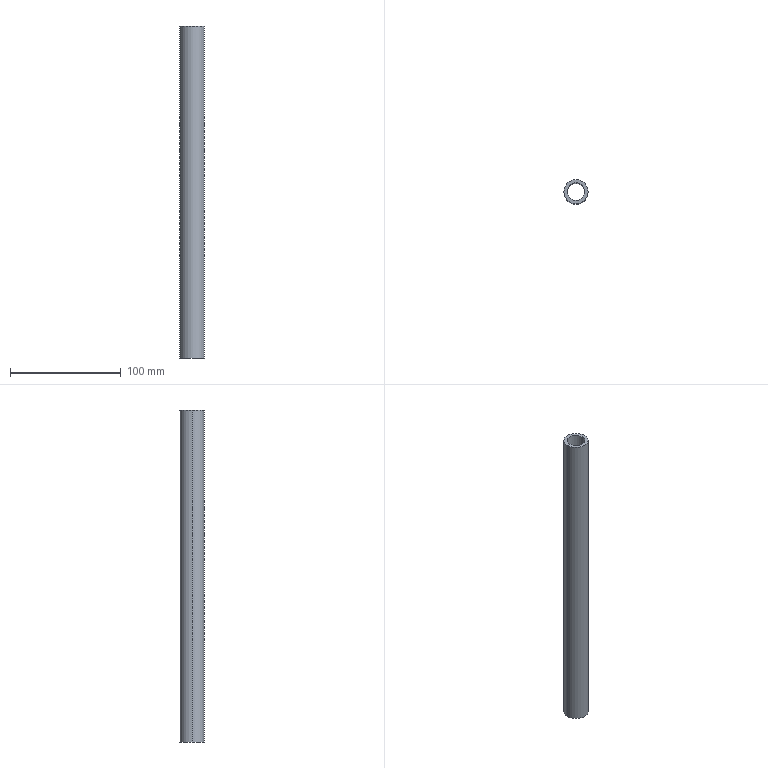Part | STEP file | 51E-01164JG10 | 1 solid | 6 faces | box 22 x 22 x 300 mm | volume 53721 mm3 | cylinder 4 | plane 2 | commonest cylinder face diameters 16 x2 22 x2
STEP:
#1=CARTESIAN_POINT('',(-8.,0.,150.));
#2=VERTEX_POINT('',#1);
#3=CARTESIAN_POINT('',(8.,0.,150.));
#4=VERTEX_POINT('',#3);
#5=CARTESIAN_POINT('',(0.,0.,150.));
#6=DIRECTION('',(0.,0.,-1.));
#7=AXIS2_PLACEMENT_3D('',#5,#6,$);
#8=CIRCLE('',#7,8.);
#9=EDGE_CURVE('',#2,#4,#8,.F.);
#10=ORIENTED_EDGE('',*,*,#9,.T.);
#11=CARTESIAN_POINT('',(8.,0.,-150.));
#12=VERTEX_POINT('',#11);
#13=CARTESIAN_POINT('',(8.,0.,150.));
#14=DIRECTION('',(0.,0.,-1.));
#15=VECTOR('',#14,1.);
#16=LINE('',#13,#15);
#17=EDGE_CURVE('',#4,#12,#16,.T.);
#18=ORIENTED_EDGE('',*,*,#17,.T.);
#19=CARTESIAN_POINT('',(-8.,0.,-150.));
#20=VERTEX_POINT('',#19);
#21=CARTESIAN_POINT('',(0.,0.,-150.));
#22=DIRECTION('',(0.,0.,-1.));
#23=AXIS2_PLACEMENT_3D('',#21,#22,$);
#24=CIRCLE('',#23,8.);
#25=EDGE_CURVE('',#20,#12,#24,.F.);
#26=ORIENTED_EDGE('',*,*,#25,.F.);
#27=CARTESIAN_POINT('',(-8.,0.,150.));
#28=DIRECTION('',(0.,0.,-1.));
#29=VECTOR('',#28,1.);
#30=LINE('',#27,#29);
#31=EDGE_CURVE('',#2,#20,#30,.T.);
#32=ORIENTED_EDGE('',*,*,#31,.F.);
#33=EDGE_LOOP('',(#10,#18,#26,#32));
#34=FACE_OUTER_BOUND('',#33,.T.);
#35=CARTESIAN_POINT('',(0.,0.,150.));
#36=DIRECTION('',(0.,0.,-1.));
#37=DIRECTION('',(1.,0.,0.));
#38=AXIS2_PLACEMENT_3D('',#35,#36,#37);
#39=CYLINDRICAL_SURFACE('',#38,8.);
#40=ADVANCED_FACE('',(#34),#39,.F.);
#41=CARTESIAN_POINT('',(-11.,0.,150.));
#42=VERTEX_POINT('',#41);
#43=CARTESIAN_POINT('',(11.,0.,150.));
#44=VERTEX_POINT('',#43);
#45=CARTESIAN_POINT('',(0.,0.,150.));
#46=DIRECTION('',(0.,0.,1.));
#47=AXIS2_PLACEMENT_3D('',#45,#46,$);
#48=CIRCLE('',#47,11.);
#49=EDGE_CURVE('',#42,#44,#48,.T.);
#50=ORIENTED_EDGE('',*,*,#49,.T.);
#51=CARTESIAN_POINT('',(0.,0.,150.));
#52=DIRECTION('',(0.,0.,1.));
#53=AXIS2_PLACEMENT_3D('',#51,#52,$);
#54=CIRCLE('',#53,11.);
#55=EDGE_CURVE('',#44,#42,#54,.T.);
#56=ORIENTED_EDGE('',*,*,#55,.T.);
#57=EDGE_LOOP('',(#50,#56));
#58=FACE_OUTER_BOUND('',#57,.T.);
#59=ORIENTED_EDGE('',*,*,#9,.F.);
#60=CARTESIAN_POINT('',(0.,0.,150.));
#61=DIRECTION('',(0.,0.,1.));
#62=AXIS2_PLACEMENT_3D('',#60,#61,$);
#63=CIRCLE('',#62,8.);
#64=EDGE_CURVE('',#4,#2,#63,.T.);
#65=ORIENTED_EDGE('',*,*,#64,.F.);
#66=EDGE_LOOP('',(#59,#65));
#67=FACE_BOUND('',#66,.T.);
#68=CARTESIAN_POINT('',(0.,0.,150.));
#69=DIRECTION('',(0.,0.,1.));
#70=DIRECTION('',(1.,0.,0.));
#71=AXIS2_PLACEMENT_3D('',#68,#69,#70);
#72=PLANE('',#71);
#73=ADVANCED_FACE('',(#58,#67),#72,.T.);
#74=ORIENTED_EDGE('',*,*,#17,.F.);
#75=ORIENTED_EDGE('',*,*,#64,.T.);
#76=ORIENTED_EDGE('',*,*,#31,.T.);
#77=CARTESIAN_POINT('',(0.,0.,-150.));
#78=DIRECTION('',(0.,0.,-1.));
#79=AXIS2_PLACEMENT_3D('',#77,#78,$);
#80=CIRCLE('',#79,8.);
#81=EDGE_CURVE('',#12,#20,#80,.F.);
#82=ORIENTED_EDGE('',*,*,#81,.F.);
#83=EDGE_LOOP('',(#74,#75,#76,#82));
#84=FACE_OUTER_BOUND('',#83,.T.);
#85=CARTESIAN_POINT('',(0.,0.,150.));
#86=DIRECTION('',(0.,0.,-1.));
#87=DIRECTION('',(-1.,0.,0.));
#88=AXIS2_PLACEMENT_3D('',#85,#86,#87);
#89=CYLINDRICAL_SURFACE('',#88,8.);
#90=ADVANCED_FACE('',(#84),#89,.F.);
#91=CARTESIAN_POINT('',(-11.,0.,-150.));
#92=VERTEX_POINT('',#91);
#93=CARTESIAN_POINT('',(11.,0.,-150.));
#94=VERTEX_POINT('',#93);
#95=CARTESIAN_POINT('',(0.,0.,-150.));
#96=DIRECTION('',(0.,0.,1.));
#97=AXIS2_PLACEMENT_3D('',#95,#96,$);
#98=CIRCLE('',#97,11.);
#99=EDGE_CURVE('',#92,#94,#98,.T.);
#100=ORIENTED_EDGE('',*,*,#99,.F.);
#101=CARTESIAN_POINT('',(0.,0.,-150.));
#102=DIRECTION('',(0.,0.,1.));
#103=AXIS2_PLACEMENT_3D('',#101,#102,$);
#104=CIRCLE('',#103,11.);
#105=EDGE_CURVE('',#94,#92,#104,.T.);
#106=ORIENTED_EDGE('',*,*,#105,.F.);
#107=EDGE_LOOP('',(#100,#106));
#108=FACE_OUTER_BOUND('',#107,.T.);
#109=ORIENTED_EDGE('',*,*,#25,.T.);
#110=ORIENTED_EDGE('',*,*,#81,.T.);
#111=EDGE_LOOP('',(#109,#110));
#112=FACE_BOUND('',#111,.T.);
#113=CARTESIAN_POINT('',(0.,0.,-150.));
#114=DIRECTION('',(0.,0.,1.));
#115=DIRECTION('',(1.,0.,0.));
#116=AXIS2_PLACEMENT_3D('',#113,#114,#115);
#117=PLANE('',#116);
#118=ADVANCED_FACE('',(#108,#112),#117,.F.);
#119=CARTESIAN_POINT('',(11.,0.,150.));
#120=DIRECTION('',(0.,0.,-1.));
#121=VECTOR('',#120,1.);
#122=LINE('',#119,#121);
#123=EDGE_CURVE('',#44,#94,#122,.T.);
#124=ORIENTED_EDGE('',*,*,#123,.F.);
#125=ORIENTED_EDGE('',*,*,#49,.F.);
#126=CARTESIAN_POINT('',(-11.,0.,150.));
#127=DIRECTION('',(0.,0.,-1.));
#128=VECTOR('',#127,1.);
#129=LINE('',#126,#128);
#130=EDGE_CURVE('',#42,#92,#129,.T.);
#131=ORIENTED_EDGE('',*,*,#130,.T.);
#132=ORIENTED_EDGE('',*,*,#99,.T.);
#133=EDGE_LOOP('',(#124,#125,#131,#132));
#134=FACE_OUTER_BOUND('',#133,.T.);
#135=CARTESIAN_POINT('',(0.,0.,150.));
#136=DIRECTION('',(0.,0.,-1.));
#137=DIRECTION('',(1.,0.,0.));
#138=AXIS2_PLACEMENT_3D('',#135,#136,#137);
#139=CYLINDRICAL_SURFACE('',#138,11.);
#140=ADVANCED_FACE('',(#134),#139,.T.);
#141=ORIENTED_EDGE('',*,*,#55,.F.);
#142=ORIENTED_EDGE('',*,*,#123,.T.);
#143=ORIENTED_EDGE('',*,*,#105,.T.);
#144=ORIENTED_EDGE('',*,*,#130,.F.);
#145=EDGE_LOOP('',(#141,#142,#143,#144));
#146=FACE_OUTER_BOUND('',#145,.T.);
#147=CARTESIAN_POINT('',(0.,0.,150.));
#148=DIRECTION('',(0.,0.,-1.));
#149=DIRECTION('',(-1.,0.,0.));
#150=AXIS2_PLACEMENT_3D('',#147,#148,#149);
#151=CYLINDRICAL_SURFACE('',#150,11.);
#152=ADVANCED_FACE('',(#146),#151,.T.);
#153=CLOSED_SHELL('',(#40,#73,#90,#118,#140,#152));
#154=MANIFOLD_SOLID_BREP('',#153);
#155=(LENGTH_UNIT()NAMED_UNIT(*)SI_UNIT(.MILLI.,.METRE.));
#156=UNCERTAINTY_MEASURE_WITH_UNIT(LENGTH_MEASURE(0.005),#155,'','');
#157=(NAMED_UNIT(*)PLANE_ANGLE_UNIT()SI_UNIT($,.RADIAN.));
#158=(NAMED_UNIT(*)SI_UNIT($,.STERADIAN.)SOLID_ANGLE_UNIT());
#159=(GEOMETRIC_REPRESENTATION_CONTEXT(3)GLOBAL_UNCERTAINTY_ASSIGNED_CONTEXT((#156))GLOBAL_UNIT_ASSIGNED_CONTEXT((#155,#157,#158))REPRESENTATION_CONTEXT('',''));
#160=ADVANCED_BREP_SHAPE_REPRESENTATION('',(#154),#159);